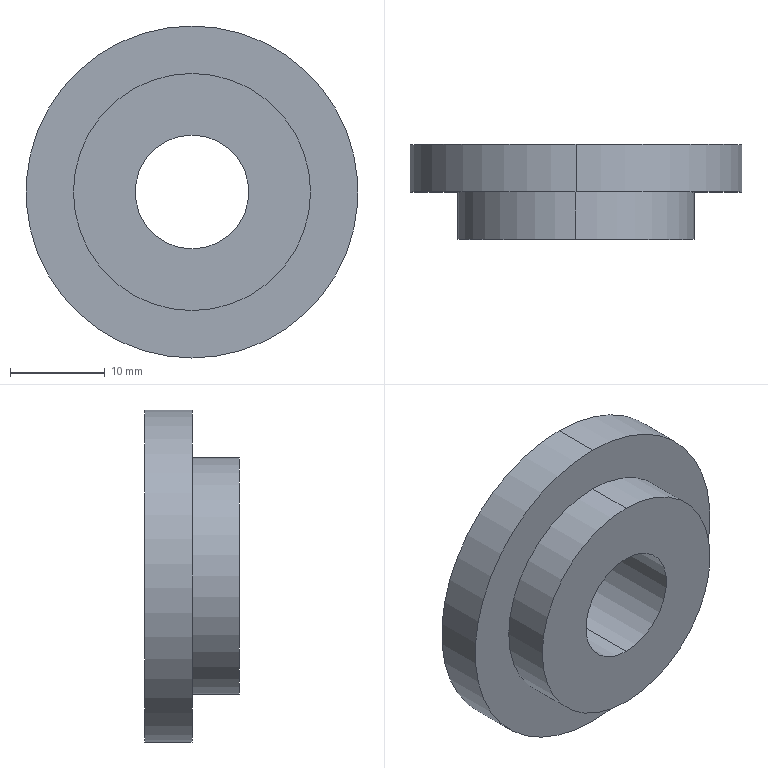Part | SolidWorks | features BaseBody 1 | 1 solid | 9 faces | box 35 x 10 x 35 mm | volume 6134 mm3 | cylinder 6 | plane 3 | commonest cylinder face diameters 12 x2 25 x2 35 x2
STEP:
#1=CARTESIAN_POINT('',(0.,5.,6.));
#2=VERTEX_POINT('',#1);
#3=CARTESIAN_POINT('',(0.,5.,-6.));
#4=VERTEX_POINT('',#3);
#5=CARTESIAN_POINT('',(0.,5.,0.));
#6=DIRECTION('',(0.,-1.,0.));
#7=DIRECTION('',(0.,0.,-1.));
#8=AXIS2_PLACEMENT_3D('',#5,#6,#7);
#9=CIRCLE('',#8,6.);
#10=EDGE_CURVE('',#2,#4,#9,.T.);
#11=ORIENTED_EDGE('',*,*,#10,.F.);
#12=CARTESIAN_POINT('',(0.,-5.,6.));
#13=VERTEX_POINT('',#12);
#14=CARTESIAN_POINT('',(0.,5.,6.));
#15=DIRECTION('',(0.,-1.,0.));
#16=VECTOR('',#15,1000.);
#17=LINE('',#14,#16);
#18=EDGE_CURVE('',#2,#13,#17,.T.);
#19=ORIENTED_EDGE('',*,*,#18,.T.);
#20=CARTESIAN_POINT('',(0.,-5.,-6.));
#21=VERTEX_POINT('',#20);
#22=CARTESIAN_POINT('',(0.,-5.,0.));
#23=DIRECTION('',(0.,1.,0.));
#24=DIRECTION('',(0.,0.,-1.));
#25=AXIS2_PLACEMENT_3D('',#22,#23,#24);
#26=CIRCLE('',#25,6.);
#27=EDGE_CURVE('',#21,#13,#26,.T.);
#28=ORIENTED_EDGE('',*,*,#27,.F.);
#29=CARTESIAN_POINT('',(0.,5.,-6.));
#30=DIRECTION('',(0.,-1.,0.));
#31=VECTOR('',#30,1000.);
#32=LINE('',#29,#31);
#33=EDGE_CURVE('',#4,#21,#32,.T.);
#34=ORIENTED_EDGE('',*,*,#33,.F.);
#35=EDGE_LOOP('',(#11,#19,#28,#34));
#36=FACE_OUTER_BOUND('',#35,.T.);
#37=CARTESIAN_POINT('',(0.,5.,0.));
#38=DIRECTION('',(0.,-1.,0.));
#39=DIRECTION('',(0.,0.,-1.));
#40=AXIS2_PLACEMENT_3D('',#37,#38,#39);
#41=CYLINDRICAL_SURFACE('',#40,6.);
#42=ADVANCED_FACE('',(#36),#41,.F.);
#43=CARTESIAN_POINT('',(0.,5.,17.5));
#44=VERTEX_POINT('',#43);
#45=CARTESIAN_POINT('',(0.,5.,-17.5));
#46=VERTEX_POINT('',#45);
#47=CARTESIAN_POINT('',(0.,5.,0.));
#48=DIRECTION('',(0.,1.,0.));
#49=DIRECTION('',(0.,0.,-1.));
#50=AXIS2_PLACEMENT_3D('',#47,#48,#49);
#51=CIRCLE('',#50,17.5);
#52=EDGE_CURVE('',#44,#46,#51,.T.);
#53=ORIENTED_EDGE('',*,*,#52,.F.);
#54=CARTESIAN_POINT('',(0.,0.,17.5));
#55=VERTEX_POINT('',#54);
#56=CARTESIAN_POINT('',(0.,5.,17.5));
#57=DIRECTION('',(0.,-1.,0.));
#58=VECTOR('',#57,1000.);
#59=LINE('',#56,#58);
#60=EDGE_CURVE('',#44,#55,#59,.T.);
#61=ORIENTED_EDGE('',*,*,#60,.T.);
#62=CARTESIAN_POINT('',(0.,0.,-17.5));
#63=VERTEX_POINT('',#62);
#64=CARTESIAN_POINT('',(0.,0.,0.));
#65=DIRECTION('',(0.,1.,0.));
#66=DIRECTION('',(0.,0.,-1.));
#67=AXIS2_PLACEMENT_3D('',#64,#65,#66);
#68=CIRCLE('',#67,17.5);
#69=EDGE_CURVE('',#55,#63,#68,.T.);
#70=ORIENTED_EDGE('',*,*,#69,.T.);
#71=CARTESIAN_POINT('',(0.,5.,-17.5));
#72=DIRECTION('',(0.,-1.,0.));
#73=VECTOR('',#72,1000.);
#74=LINE('',#71,#73);
#75=EDGE_CURVE('',#46,#63,#74,.T.);
#76=ORIENTED_EDGE('',*,*,#75,.F.);
#77=EDGE_LOOP('',(#53,#61,#70,#76));
#78=FACE_OUTER_BOUND('',#77,.T.);
#79=CARTESIAN_POINT('',(0.,5.,0.));
#80=DIRECTION('',(0.,-1.,0.));
#81=DIRECTION('',(0.,0.,-1.));
#82=AXIS2_PLACEMENT_3D('',#79,#80,#81);
#83=CYLINDRICAL_SURFACE('',#82,17.5);
#84=ADVANCED_FACE('',(#78),#83,.T.);
#85=CARTESIAN_POINT('',(0.,-5.,-12.5));
#86=VERTEX_POINT('',#85);
#87=CARTESIAN_POINT('',(0.,-5.,12.5));
#88=VERTEX_POINT('',#87);
#89=CARTESIAN_POINT('',(0.,-5.,0.));
#90=DIRECTION('',(0.,-1.,0.));
#91=DIRECTION('',(0.,0.,1.));
#92=AXIS2_PLACEMENT_3D('',#89,#90,#91);
#93=CIRCLE('',#92,12.5);
#94=EDGE_CURVE('',#86,#88,#93,.T.);
#95=ORIENTED_EDGE('',*,*,#94,.F.);
#96=CARTESIAN_POINT('',(0.,0.,-12.5));
#97=VERTEX_POINT('',#96);
#98=CARTESIAN_POINT('',(0.,-5.,-12.5));
#99=DIRECTION('',(0.,1.,0.));
#100=VECTOR('',#99,1000.);
#101=LINE('',#98,#100);
#102=EDGE_CURVE('',#86,#97,#101,.T.);
#103=ORIENTED_EDGE('',*,*,#102,.T.);
#104=CARTESIAN_POINT('',(0.,0.,12.5));
#105=VERTEX_POINT('',#104);
#106=CARTESIAN_POINT('',(0.,0.,0.));
#107=DIRECTION('',(0.,-1.,0.));
#108=DIRECTION('',(0.,0.,1.));
#109=AXIS2_PLACEMENT_3D('',#106,#107,#108);
#110=CIRCLE('',#109,12.5);
#111=EDGE_CURVE('',#97,#105,#110,.T.);
#112=ORIENTED_EDGE('',*,*,#111,.T.);
#113=CARTESIAN_POINT('',(0.,-5.,12.5));
#114=DIRECTION('',(0.,1.,0.));
#115=VECTOR('',#114,1000.);
#116=LINE('',#113,#115);
#117=EDGE_CURVE('',#88,#105,#116,.T.);
#118=ORIENTED_EDGE('',*,*,#117,.F.);
#119=EDGE_LOOP('',(#95,#103,#112,#118));
#120=FACE_OUTER_BOUND('',#119,.T.);
#121=CARTESIAN_POINT('',(0.,-5.,0.));
#122=DIRECTION('',(0.,1.,0.));
#123=DIRECTION('',(0.,0.,1.));
#124=AXIS2_PLACEMENT_3D('',#121,#122,#123);
#125=CYLINDRICAL_SURFACE('',#124,12.5);
#126=ADVANCED_FACE('',(#120),#125,.T.);
#127=CARTESIAN_POINT('',(0.,5.,0.));
#128=DIRECTION('',(0.,-1.,0.));
#129=DIRECTION('',(0.,0.,-1.));
#130=AXIS2_PLACEMENT_3D('',#127,#128,#129);
#131=CIRCLE('',#130,6.);
#132=EDGE_CURVE('',#4,#2,#131,.T.);
#133=ORIENTED_EDGE('',*,*,#132,.T.);
#134=ORIENTED_EDGE('',*,*,#10,.T.);
#135=EDGE_LOOP('',(#133,#134));
#136=FACE_BOUND('',#135,.T.);
#137=CARTESIAN_POINT('',(0.,5.,0.));
#138=DIRECTION('',(0.,1.,0.));
#139=DIRECTION('',(0.,0.,-1.));
#140=AXIS2_PLACEMENT_3D('',#137,#138,#139);
#141=CIRCLE('',#140,17.5);
#142=EDGE_CURVE('',#46,#44,#141,.T.);
#143=ORIENTED_EDGE('',*,*,#142,.T.);
#144=ORIENTED_EDGE('',*,*,#52,.T.);
#145=EDGE_LOOP('',(#143,#144));
#146=FACE_OUTER_BOUND('',#145,.T.);
#147=CARTESIAN_POINT('',(0.,5.,0.));
#148=DIRECTION('',(0.,1.,0.));
#149=DIRECTION('',(0.,0.,1.));
#150=AXIS2_PLACEMENT_3D('',#147,#148,#149);
#151=PLANE('',#150);
#152=ADVANCED_FACE('',(#136,#146),#151,.T.);
#153=ORIENTED_EDGE('',*,*,#18,.F.);
#154=ORIENTED_EDGE('',*,*,#132,.F.);
#155=ORIENTED_EDGE('',*,*,#33,.T.);
#156=CARTESIAN_POINT('',(0.,-5.,0.));
#157=DIRECTION('',(0.,1.,0.));
#158=DIRECTION('',(0.,0.,-1.));
#159=AXIS2_PLACEMENT_3D('',#156,#157,#158);
#160=CIRCLE('',#159,6.);
#161=EDGE_CURVE('',#13,#21,#160,.T.);
#162=ORIENTED_EDGE('',*,*,#161,.F.);
#163=EDGE_LOOP('',(#153,#154,#155,#162));
#164=FACE_OUTER_BOUND('',#163,.T.);
#165=CARTESIAN_POINT('',(0.,5.,0.));
#166=DIRECTION('',(0.,-1.,0.));
#167=DIRECTION('',(0.,0.,-1.));
#168=AXIS2_PLACEMENT_3D('',#165,#166,#167);
#169=CYLINDRICAL_SURFACE('',#168,6.);
#170=ADVANCED_FACE('',(#164),#169,.F.);
#171=ORIENTED_EDGE('',*,*,#60,.F.);
#172=ORIENTED_EDGE('',*,*,#142,.F.);
#173=ORIENTED_EDGE('',*,*,#75,.T.);
#174=CARTESIAN_POINT('',(0.,0.,0.));
#175=DIRECTION('',(0.,1.,0.));
#176=DIRECTION('',(0.,0.,-1.));
#177=AXIS2_PLACEMENT_3D('',#174,#175,#176);
#178=CIRCLE('',#177,17.5);
#179=EDGE_CURVE('',#63,#55,#178,.T.);
#180=ORIENTED_EDGE('',*,*,#179,.T.);
#181=EDGE_LOOP('',(#171,#172,#173,#180));
#182=FACE_OUTER_BOUND('',#181,.T.);
#183=CARTESIAN_POINT('',(0.,5.,0.));
#184=DIRECTION('',(0.,-1.,0.));
#185=DIRECTION('',(0.,0.,-1.));
#186=AXIS2_PLACEMENT_3D('',#183,#184,#185);
#187=CYLINDRICAL_SURFACE('',#186,17.5);
#188=ADVANCED_FACE('',(#182),#187,.T.);
#189=ORIENTED_EDGE('',*,*,#27,.T.);
#190=ORIENTED_EDGE('',*,*,#161,.T.);
#191=EDGE_LOOP('',(#189,#190));
#192=FACE_BOUND('',#191,.T.);
#193=CARTESIAN_POINT('',(0.,-5.,0.));
#194=DIRECTION('',(0.,-1.,0.));
#195=DIRECTION('',(0.,0.,1.));
#196=AXIS2_PLACEMENT_3D('',#193,#194,#195);
#197=CIRCLE('',#196,12.5);
#198=EDGE_CURVE('',#88,#86,#197,.T.);
#199=ORIENTED_EDGE('',*,*,#198,.T.);
#200=ORIENTED_EDGE('',*,*,#94,.T.);
#201=EDGE_LOOP('',(#199,#200));
#202=FACE_OUTER_BOUND('',#201,.T.);
#203=CARTESIAN_POINT('',(0.,-5.,0.));
#204=DIRECTION('',(0.,-1.,0.));
#205=DIRECTION('',(0.,0.,-1.));
#206=AXIS2_PLACEMENT_3D('',#203,#204,#205);
#207=PLANE('',#206);
#208=ADVANCED_FACE('',(#192,#202),#207,.T.);
#209=CARTESIAN_POINT('',(0.,0.,0.));
#210=DIRECTION('',(0.,-1.,0.));
#211=DIRECTION('',(0.,0.,1.));
#212=AXIS2_PLACEMENT_3D('',#209,#210,#211);
#213=CIRCLE('',#212,12.5);
#214=EDGE_CURVE('',#105,#97,#213,.T.);
#215=ORIENTED_EDGE('',*,*,#214,.F.);
#216=ORIENTED_EDGE('',*,*,#111,.F.);
#217=EDGE_LOOP('',(#215,#216));
#218=FACE_BOUND('',#217,.T.);
#219=ORIENTED_EDGE('',*,*,#179,.F.);
#220=ORIENTED_EDGE('',*,*,#69,.F.);
#221=EDGE_LOOP('',(#219,#220));
#222=FACE_OUTER_BOUND('',#221,.T.);
#223=CARTESIAN_POINT('',(0.,0.,0.));
#224=DIRECTION('',(0.,1.,0.));
#225=DIRECTION('',(0.,0.,1.));
#226=AXIS2_PLACEMENT_3D('',#223,#224,#225);
#227=PLANE('',#226);
#228=ADVANCED_FACE('',(#218,#222),#227,.F.);
#229=ORIENTED_EDGE('',*,*,#102,.F.);
#230=ORIENTED_EDGE('',*,*,#198,.F.);
#231=ORIENTED_EDGE('',*,*,#117,.T.);
#232=ORIENTED_EDGE('',*,*,#214,.T.);
#233=EDGE_LOOP('',(#229,#230,#231,#232));
#234=FACE_OUTER_BOUND('',#233,.T.);
#235=CARTESIAN_POINT('',(0.,-5.,0.));
#236=DIRECTION('',(0.,1.,0.));
#237=DIRECTION('',(0.,0.,1.));
#238=AXIS2_PLACEMENT_3D('',#235,#236,#237);
#239=CYLINDRICAL_SURFACE('',#238,12.5);
#240=ADVANCED_FACE('',(#234),#239,.T.);
#241=CLOSED_SHELL('',(#42,#84,#126,#152,#170,#188,#208,#228,#240));
#242=MANIFOLD_SOLID_BREP('',#241);
#243=CARTESIAN_POINT('',(0.,0.,0.));
#244=DIRECTION('',(0.,0.,1.));
#245=DIRECTION('',(1.,0.,0.));
#246=AXIS2_PLACEMENT_3D('',#243,#244,#245);
#247=(LENGTH_UNIT()NAMED_UNIT(*)SI_UNIT(.MILLI.,.METRE.));
#248=UNCERTAINTY_MEASURE_WITH_UNIT(LENGTH_MEASURE(0.00001),#247,'','');
#249=(NAMED_UNIT(*)PLANE_ANGLE_UNIT()SI_UNIT($,.RADIAN.));
#250=(NAMED_UNIT(*)SI_UNIT($,.STERADIAN.)SOLID_ANGLE_UNIT());
#251=(GEOMETRIC_REPRESENTATION_CONTEXT(3)GLOBAL_UNCERTAINTY_ASSIGNED_CONTEXT((#248))GLOBAL_UNIT_ASSIGNED_CONTEXT((#247,#249,#250))REPRESENTATION_CONTEXT('',''));
#252=ADVANCED_BREP_SHAPE_REPRESENTATION('',(#242,#246),#251);